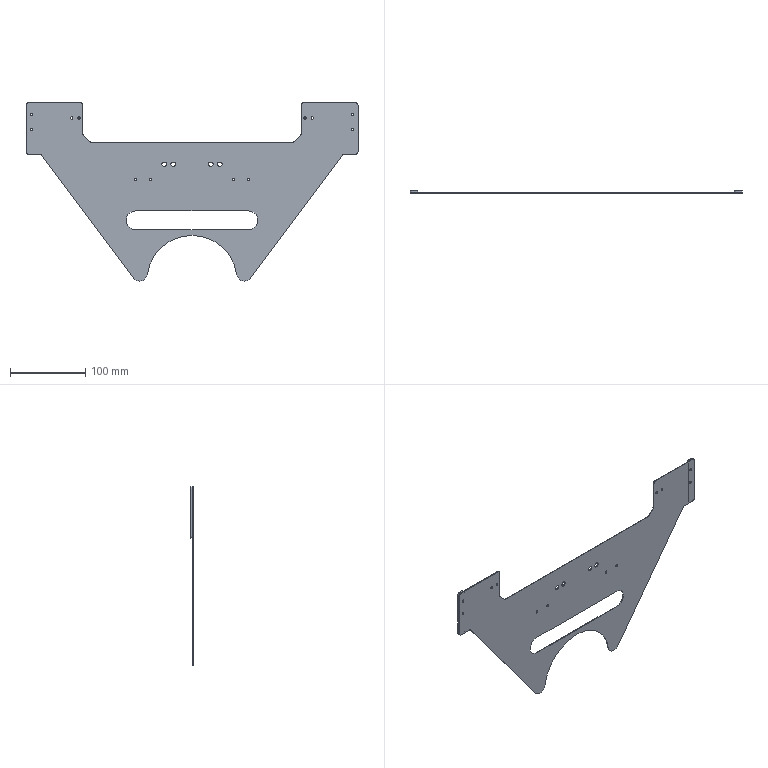Part | SolidWorks | features ICE 2, Extrusion 1, Fillet 1, MirrorSolid 1 | 3 solids | 96 faces | box 441.1 x 3 x 236.71 mm | volume 53782 mm3 | cylinder 67 | plane 29 | commonest cylinder face diameters 3.2 x32 6 x28 20 x4 25 x2 120 x1